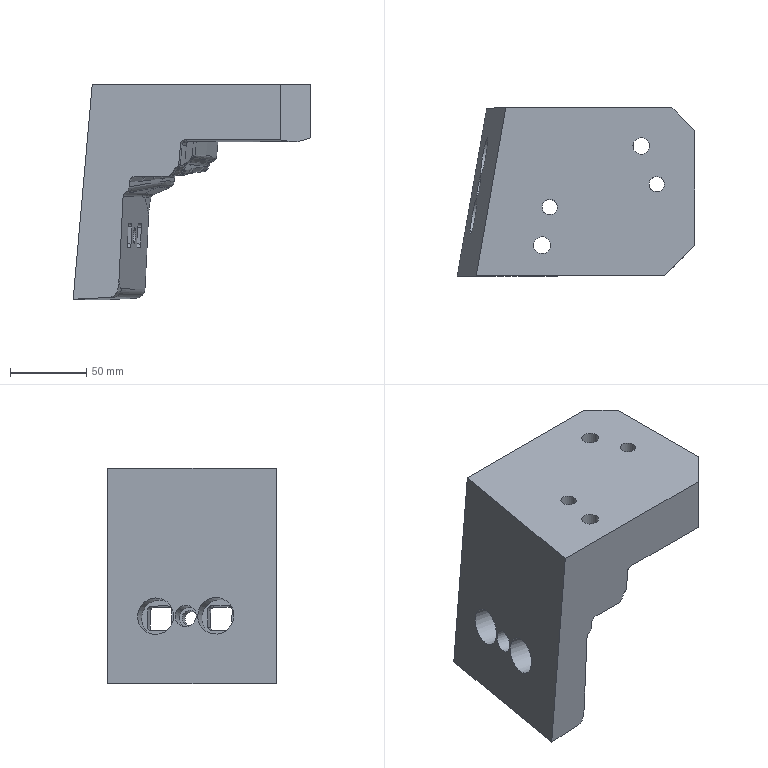Part | NX | features solid 2 | 1 solid | 120 faces | box 155.596 x 110.001 x 141.24 mm | volume 860485 mm3 | spline 56 | cylinder 40 | plane 24 | commonest cylinder face diameters 5.1 x8 10 x3 6.001 x2 6.003 x2 8.003 x2 11 x2